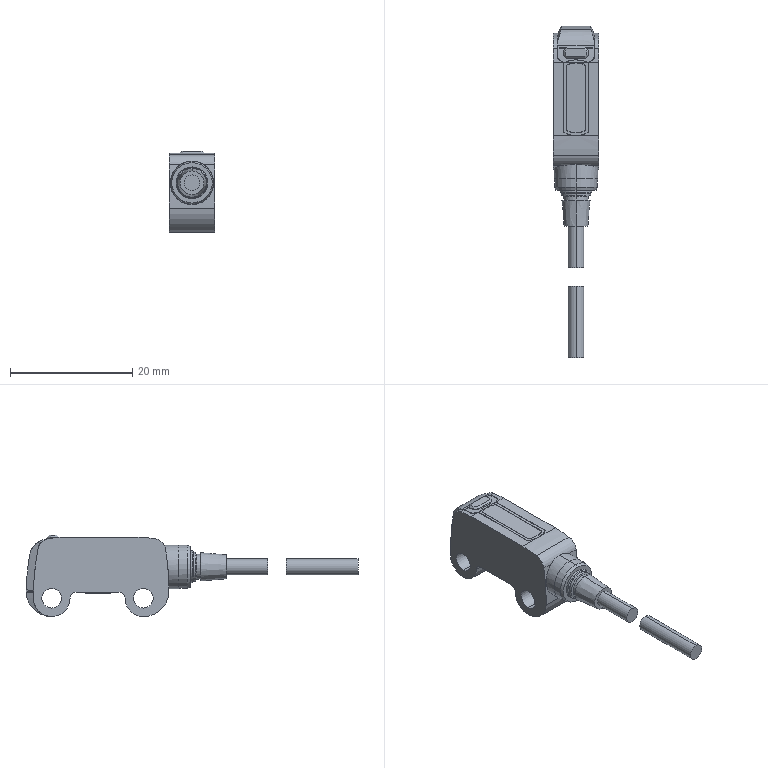Part | SolidWorks | features BaseBody 2 | 2 solids | 144 faces | box 7.5 x 54.319 x 13.3 mm | volume 2039 mm3 | cylinder 63 | plane 60 | cone 20 | spline 1 | commonest cylinder face diameters 4 x9 2.6 x4 3.2 x4 42.147 x4 86 x4 0.6 x3